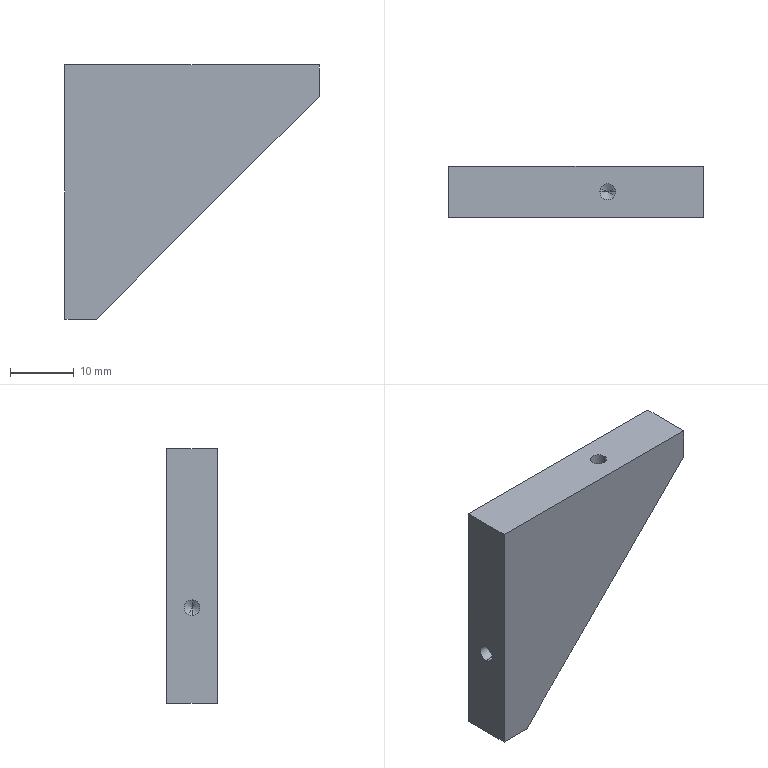Part | STEP file | PN_0010 | 1 solid | 15 faces | box 40 x 8 x 40 mm | volume 7824 mm3 | plane 7 | cylinder 4 | cone 4 | commonest cylinder face diameters 2.5 x4
STEP:
#1=CARTESIAN_POINT('',(0.,0.,0.));
#2=DIRECTION('',(0.,0.,1.));
#3=DIRECTION('',(1.,0.,0.));
#4=AXIS2_PLACEMENT_3D('',#1,#2,#3);
#5=CARTESIAN_POINT('',(-12.5,4.,-3.75));
#6=VERTEX_POINT('',#5);
#7=CARTESIAN_POINT('',(-20.,4.,-3.75));
#8=VERTEX_POINT('',#7);
#9=CARTESIAN_POINT('',(-20.,4.,-3.75));
#10=DIRECTION('',(-1.,0.,0.));
#11=VECTOR('',#10,1.);
#12=LINE('',#9,#11);
#13=CARTESIAN_POINT('',(-20.,4.,-5.));
#14=DIRECTION('',(-1.,0.,0.));
#15=DIRECTION('',(0.,0.,1.));
#16=AXIS2_PLACEMENT_3D('',#13,#14,#15);
#17=CYLINDRICAL_SURFACE('',#16,1.25);
#18=CARTESIAN_POINT('',(6.283,0.));
#19=DIRECTION('',(0.,1.));
#20=VECTOR('',#19,1.);
#21=LINE('',#18,#20);
#22=(GEOMETRIC_REPRESENTATION_CONTEXT(2)PARAMETRIC_REPRESENTATION_CONTEXT()REPRESENTATION_CONTEXT('',''));
#23=DEFINITIONAL_REPRESENTATION('',(#21),#22);
#24=PCURVE('',#17,#23);
#25=CARTESIAN_POINT('',(-20.,4.,-5.));
#26=DIRECTION('',(-1.,0.,0.));
#27=DIRECTION('',(0.,0.,1.));
#28=AXIS2_PLACEMENT_3D('',#25,#26,#27);
#29=CYLINDRICAL_SURFACE('',#28,1.25);
#30=CARTESIAN_POINT('',(0.,0.));
#31=DIRECTION('',(0.,1.));
#32=VECTOR('',#31,1.);
#33=LINE('',#30,#32);
#34=(GEOMETRIC_REPRESENTATION_CONTEXT(2)PARAMETRIC_REPRESENTATION_CONTEXT()REPRESENTATION_CONTEXT('',''));
#35=DEFINITIONAL_REPRESENTATION('',(#33),#34);
#36=PCURVE('',#29,#35);
#37=SURFACE_CURVE('',#12,(#24,#36),.PCURVE_S1.);
#38=EDGE_CURVE('',#6,#8,#37,.T.);
#39=ORIENTED_EDGE('',*,*,#38,.T.);
#40=CARTESIAN_POINT('',(-20.,4.,-6.25));
#41=VERTEX_POINT('',#40);
#42=CARTESIAN_POINT('',(-20.,4.,-5.));
#43=DIRECTION('',(-1.,0.,0.));
#44=DIRECTION('',(0.,0.,1.));
#45=AXIS2_PLACEMENT_3D('',#42,#43,#44);
#46=CIRCLE('',#45,1.25);
#47=CARTESIAN_POINT('',(0.,0.));
#48=DIRECTION('',(1.,0.));
#49=VECTOR('',#48,1.);
#50=LINE('',#47,#49);
#51=(GEOMETRIC_REPRESENTATION_CONTEXT(2)PARAMETRIC_REPRESENTATION_CONTEXT()REPRESENTATION_CONTEXT('',''));
#52=DEFINITIONAL_REPRESENTATION('',(#50),#51);
#53=PCURVE('',#17,#52);
#54=CARTESIAN_POINT('',(-20.,8.,-20.));
#55=DIRECTION('',(1.,0.,0.));
#56=DIRECTION('',(0.,0.,-1.));
#57=AXIS2_PLACEMENT_3D('',#54,#55,#56);
#58=PLANE('',#57);
#59=CARTESIAN_POINT('',(-16.25,-4.));
#60=CARTESIAN_POINT('',(-16.25,-1.835));
#61=CARTESIAN_POINT('',(-14.375,-2.917));
#62=CARTESIAN_POINT('',(-12.5,-4.));
#63=CARTESIAN_POINT('',(-14.375,-5.083));
#64=CARTESIAN_POINT('',(-16.25,-6.165));
#65=CARTESIAN_POINT('',(-16.25,-4.));
#66=(BOUNDED_CURVE()B_SPLINE_CURVE(2,(#59,#60,#61,#62,#63,#64,#65),.UNSPECIFIED.,.T.,.F.)B_SPLINE_CURVE_WITH_KNOTS((1,2,2,2,2,1),(-2.094,0.,2.094,4.189,6.283,8.378),.UNSPECIFIED.)CURVE()GEOMETRIC_REPRESENTATION_ITEM()RATIONAL_B_SPLINE_CURVE((1.,0.5,1.,0.5,1.,0.5,1.))REPRESENTATION_ITEM(''));
#67=(GEOMETRIC_REPRESENTATION_CONTEXT(2)PARAMETRIC_REPRESENTATION_CONTEXT()REPRESENTATION_CONTEXT('',''));
#68=DEFINITIONAL_REPRESENTATION('',(#66),#67);
#69=PCURVE('',#58,#68);
#70=SURFACE_CURVE('',#46,(#53,#69),.PCURVE_S1.);
#71=EDGE_CURVE('',#41,#8,#70,.T.);
#72=ORIENTED_EDGE('',*,*,#71,.F.);
#73=CARTESIAN_POINT('',(-12.5,4.,-6.25));
#74=VERTEX_POINT('',#73);
#75=CARTESIAN_POINT('',(-20.,4.,-6.25));
#76=DIRECTION('',(-1.,0.,0.));
#77=VECTOR('',#76,1.);
#78=LINE('',#75,#77);
#79=CARTESIAN_POINT('',(3.142,0.));
#80=DIRECTION('',(0.,1.));
#81=VECTOR('',#80,1.);
#82=LINE('',#79,#81);
#83=(GEOMETRIC_REPRESENTATION_CONTEXT(2)PARAMETRIC_REPRESENTATION_CONTEXT()REPRESENTATION_CONTEXT('',''));
#84=DEFINITIONAL_REPRESENTATION('',(#82),#83);
#85=PCURVE('',#17,#84);
#86=CARTESIAN_POINT('',(3.142,0.));
#87=DIRECTION('',(0.,1.));
#88=VECTOR('',#87,1.);
#89=LINE('',#86,#88);
#90=(GEOMETRIC_REPRESENTATION_CONTEXT(2)PARAMETRIC_REPRESENTATION_CONTEXT()REPRESENTATION_CONTEXT('',''));
#91=DEFINITIONAL_REPRESENTATION('',(#89),#90);
#92=PCURVE('',#29,#91);
#93=SURFACE_CURVE('',#78,(#85,#92),.PCURVE_S1.);
#94=EDGE_CURVE('',#74,#41,#93,.T.);
#95=ORIENTED_EDGE('',*,*,#94,.F.);
#96=CARTESIAN_POINT('',(-12.5,4.,-5.));
#97=DIRECTION('',(-1.,0.,0.));
#98=DIRECTION('',(0.,0.,1.));
#99=AXIS2_PLACEMENT_3D('',#96,#97,#98);
#100=CIRCLE('',#99,1.25);
#101=CARTESIAN_POINT('',(0.,-7.5));
#102=DIRECTION('',(1.,0.));
#103=VECTOR('',#102,1.);
#104=LINE('',#101,#103);
#105=(GEOMETRIC_REPRESENTATION_CONTEXT(2)PARAMETRIC_REPRESENTATION_CONTEXT()REPRESENTATION_CONTEXT('',''));
#106=DEFINITIONAL_REPRESENTATION('',(#104),#105);
#107=PCURVE('',#17,#106);
#108=CARTESIAN_POINT('',(-12.5,4.,-5.));
#109=DIRECTION('',(-1.,0.,0.));
#110=DIRECTION('',(0.,0.,1.));
#111=AXIS2_PLACEMENT_3D('',#108,#109,#110);
#112=CONICAL_SURFACE('',#111,1.25,1.03);
#113=CARTESIAN_POINT('',(0.,0.));
#114=DIRECTION('',(1.,0.));
#115=VECTOR('',#114,1.);
#116=LINE('',#113,#115);
#117=(GEOMETRIC_REPRESENTATION_CONTEXT(2)PARAMETRIC_REPRESENTATION_CONTEXT()REPRESENTATION_CONTEXT('',''));
#118=DEFINITIONAL_REPRESENTATION('',(#116),#117);
#119=PCURVE('',#112,#118);
#120=SURFACE_CURVE('',#100,(#107,#119),.PCURVE_S1.);
#121=EDGE_CURVE('',#74,#6,#120,.T.);
#122=ORIENTED_EDGE('',*,*,#121,.T.);
#123=EDGE_LOOP('',(#39,#72,#95,#122));
#124=FACE_BOUND('',#123,.F.);
#125=ADVANCED_FACE('',(#124),#17,.F.);
#126=ORIENTED_EDGE('',*,*,#121,.F.);
#127=CARTESIAN_POINT('',(-11.749,4.,-5.));
#128=VERTEX_POINT('',#127);
#129=CARTESIAN_POINT('',(-12.5,4.,-6.25));
#130=DIRECTION('',(-0.515,0.,-0.8572));
#131=VECTOR('',#130,1.);
#132=LINE('',#129,#131);
#133=CARTESIAN_POINT('',(3.142,0.));
#134=DIRECTION('',(0.,1.));
#135=VECTOR('',#134,1.);
#136=LINE('',#133,#135);
#137=(GEOMETRIC_REPRESENTATION_CONTEXT(2)PARAMETRIC_REPRESENTATION_CONTEXT()REPRESENTATION_CONTEXT('',''));
#138=DEFINITIONAL_REPRESENTATION('',(#136),#137);
#139=PCURVE('',#112,#138);
#140=CARTESIAN_POINT('',(-12.5,4.,-5.));
#141=DIRECTION('',(-1.,0.,0.));
#142=DIRECTION('',(0.,0.,1.));
#143=AXIS2_PLACEMENT_3D('',#140,#141,#142);
#144=CONICAL_SURFACE('',#143,1.25,1.03);
#145=CARTESIAN_POINT('',(3.142,0.));
#146=DIRECTION('',(0.,1.));
#147=VECTOR('',#146,1.);
#148=LINE('',#145,#147);
#149=(GEOMETRIC_REPRESENTATION_CONTEXT(2)PARAMETRIC_REPRESENTATION_CONTEXT()REPRESENTATION_CONTEXT('',''));
#150=DEFINITIONAL_REPRESENTATION('',(#148),#149);
#151=PCURVE('',#144,#150);
#152=SURFACE_CURVE('',#132,(#139,#151),.PCURVE_S1.);
#153=EDGE_CURVE('',#128,#74,#152,.T.);
#154=ORIENTED_EDGE('',*,*,#153,.F.);
#155=CARTESIAN_POINT('',(-12.5,4.,-3.75));
#156=DIRECTION('',(-0.515,0.,0.8572));
#157=VECTOR('',#156,1.);
#158=LINE('',#155,#157);
#159=CARTESIAN_POINT('',(6.283,0.));
#160=DIRECTION('',(0.,1.));
#161=VECTOR('',#160,1.);
#162=LINE('',#159,#161);
#163=(GEOMETRIC_REPRESENTATION_CONTEXT(2)PARAMETRIC_REPRESENTATION_CONTEXT()REPRESENTATION_CONTEXT('',''));
#164=DEFINITIONAL_REPRESENTATION('',(#162),#163);
#165=PCURVE('',#112,#164);
#166=CARTESIAN_POINT('',(0.,0.));
#167=DIRECTION('',(0.,1.));
#168=VECTOR('',#167,1.);
#169=LINE('',#166,#168);
#170=(GEOMETRIC_REPRESENTATION_CONTEXT(2)PARAMETRIC_REPRESENTATION_CONTEXT()REPRESENTATION_CONTEXT('',''));
#171=DEFINITIONAL_REPRESENTATION('',(#169),#170);
#172=PCURVE('',#144,#171);
#173=SURFACE_CURVE('',#158,(#165,#172),.PCURVE_S1.);
#174=EDGE_CURVE('',#128,#6,#173,.T.);
#175=ORIENTED_EDGE('',*,*,#174,.T.);
#176=EDGE_LOOP('',(#126,#154,#175));
#177=FACE_BOUND('',#176,.F.);
#178=ADVANCED_FACE('',(#177),#112,.F.);
#179=CARTESIAN_POINT('',(6.25,4.,12.5));
#180=VERTEX_POINT('',#179);
#181=CARTESIAN_POINT('',(6.25,4.,20.));
#182=VERTEX_POINT('',#181);
#183=CARTESIAN_POINT('',(6.25,4.,20.));
#184=DIRECTION('',(0.,0.,1.));
#185=VECTOR('',#184,1.);
#186=LINE('',#183,#185);
#187=CARTESIAN_POINT('',(5.,4.,20.));
#188=DIRECTION('',(0.,0.,1.));
#189=DIRECTION('',(1.,0.,0.));
#190=AXIS2_PLACEMENT_3D('',#187,#188,#189);
#191=CYLINDRICAL_SURFACE('',#190,1.25);
#192=CARTESIAN_POINT('',(6.283,0.));
#193=DIRECTION('',(0.,1.));
#194=VECTOR('',#193,1.);
#195=LINE('',#192,#194);
#196=(GEOMETRIC_REPRESENTATION_CONTEXT(2)PARAMETRIC_REPRESENTATION_CONTEXT()REPRESENTATION_CONTEXT('',''));
#197=DEFINITIONAL_REPRESENTATION('',(#195),#196);
#198=PCURVE('',#191,#197);
#199=CARTESIAN_POINT('',(5.,4.,20.));
#200=DIRECTION('',(0.,0.,1.));
#201=DIRECTION('',(1.,0.,0.));
#202=AXIS2_PLACEMENT_3D('',#199,#200,#201);
#203=CYLINDRICAL_SURFACE('',#202,1.25);
#204=CARTESIAN_POINT('',(0.,0.));
#205=DIRECTION('',(0.,1.));
#206=VECTOR('',#205,1.);
#207=LINE('',#204,#206);
#208=(GEOMETRIC_REPRESENTATION_CONTEXT(2)PARAMETRIC_REPRESENTATION_CONTEXT()REPRESENTATION_CONTEXT('',''));
#209=DEFINITIONAL_REPRESENTATION('',(#207),#208);
#210=PCURVE('',#203,#209);
#211=SURFACE_CURVE('',#186,(#198,#210),.PCURVE_S1.);
#212=EDGE_CURVE('',#180,#182,#211,.T.);
#213=ORIENTED_EDGE('',*,*,#212,.T.);
#214=CARTESIAN_POINT('',(3.75,4.,20.));
#215=VERTEX_POINT('',#214);
#216=CARTESIAN_POINT('',(5.,4.,20.));
#217=DIRECTION('',(0.,0.,1.));
#218=DIRECTION('',(1.,0.,0.));
#219=AXIS2_PLACEMENT_3D('',#216,#217,#218);
#220=CIRCLE('',#219,1.25);
#221=CARTESIAN_POINT('',(0.,0.));
#222=DIRECTION('',(1.,0.));
#223=VECTOR('',#222,1.);
#224=LINE('',#221,#223);
#225=(GEOMETRIC_REPRESENTATION_CONTEXT(2)PARAMETRIC_REPRESENTATION_CONTEXT()REPRESENTATION_CONTEXT('',''));
#226=DEFINITIONAL_REPRESENTATION('',(#224),#225);
#227=PCURVE('',#191,#226);
#228=CARTESIAN_POINT('',(-20.,8.,20.));
#229=DIRECTION('',(0.,0.,-1.));
#230=DIRECTION('',(-1.,0.,0.));
#231=AXIS2_PLACEMENT_3D('',#228,#229,#230);
#232=PLANE('',#231);
#233=CARTESIAN_POINT('',(-26.25,-4.));
#234=CARTESIAN_POINT('',(-26.25,-1.835));
#235=CARTESIAN_POINT('',(-24.375,-2.917));
#236=CARTESIAN_POINT('',(-22.5,-4.));
#237=CARTESIAN_POINT('',(-24.375,-5.083));
#238=CARTESIAN_POINT('',(-26.25,-6.165));
#239=CARTESIAN_POINT('',(-26.25,-4.));
#240=(BOUNDED_CURVE()B_SPLINE_CURVE(2,(#233,#234,#235,#236,#237,#238,#239),.UNSPECIFIED.,.T.,.F.)B_SPLINE_CURVE_WITH_KNOTS((1,2,2,2,2,1),(-2.094,0.,2.094,4.189,6.283,8.378),.UNSPECIFIED.)CURVE()GEOMETRIC_REPRESENTATION_ITEM()RATIONAL_B_SPLINE_CURVE((1.,0.5,1.,0.5,1.,0.5,1.))REPRESENTATION_ITEM(''));
#241=(GEOMETRIC_REPRESENTATION_CONTEXT(2)PARAMETRIC_REPRESENTATION_CONTEXT()REPRESENTATION_CONTEXT('',''));
#242=DEFINITIONAL_REPRESENTATION('',(#240),#241);
#243=PCURVE('',#232,#242);
#244=SURFACE_CURVE('',#220,(#227,#243),.PCURVE_S1.);
#245=EDGE_CURVE('',#215,#182,#244,.T.);
#246=ORIENTED_EDGE('',*,*,#245,.F.);
#247=CARTESIAN_POINT('',(3.75,4.,12.5));
#248=VERTEX_POINT('',#247);
#249=CARTESIAN_POINT('',(3.75,4.,20.));
#250=DIRECTION('',(0.,0.,1.));
#251=VECTOR('',#250,1.);
#252=LINE('',#249,#251);
#253=CARTESIAN_POINT('',(3.142,0.));
#254=DIRECTION('',(0.,1.));
#255=VECTOR('',#254,1.);
#256=LINE('',#253,#255);
#257=(GEOMETRIC_REPRESENTATION_CONTEXT(2)PARAMETRIC_REPRESENTATION_CONTEXT()REPRESENTATION_CONTEXT('',''));
#258=DEFINITIONAL_REPRESENTATION('',(#256),#257);
#259=PCURVE('',#191,#258);
#260=CARTESIAN_POINT('',(3.142,0.));
#261=DIRECTION('',(0.,1.));
#262=VECTOR('',#261,1.);
#263=LINE('',#260,#262);
#264=(GEOMETRIC_REPRESENTATION_CONTEXT(2)PARAMETRIC_REPRESENTATION_CONTEXT()REPRESENTATION_CONTEXT('',''));
#265=DEFINITIONAL_REPRESENTATION('',(#263),#264);
#266=PCURVE('',#203,#265);
#267=SURFACE_CURVE('',#252,(#259,#266),.PCURVE_S1.);
#268=EDGE_CURVE('',#248,#215,#267,.T.);
#269=ORIENTED_EDGE('',*,*,#268,.F.);
#270=CARTESIAN_POINT('',(5.,4.,12.5));
#271=DIRECTION('',(0.,0.,1.));
#272=DIRECTION('',(1.,0.,0.));
#273=AXIS2_PLACEMENT_3D('',#270,#271,#272);
#274=CIRCLE('',#273,1.25);
#275=CARTESIAN_POINT('',(0.,-7.5));
#276=DIRECTION('',(1.,0.));
#277=VECTOR('',#276,1.);
#278=LINE('',#275,#277);
#279=(GEOMETRIC_REPRESENTATION_CONTEXT(2)PARAMETRIC_REPRESENTATION_CONTEXT()REPRESENTATION_CONTEXT('',''));
#280=DEFINITIONAL_REPRESENTATION('',(#278),#279);
#281=PCURVE('',#191,#280);
#282=CARTESIAN_POINT('',(5.,4.,12.5));
#283=DIRECTION('',(0.,0.,1.));
#284=DIRECTION('',(1.,0.,0.));
#285=AXIS2_PLACEMENT_3D('',#282,#283,#284);
#286=CONICAL_SURFACE('',#285,1.25,1.03);
#287=CARTESIAN_POINT('',(0.,0.));
#288=DIRECTION('',(1.,0.));
#289=VECTOR('',#288,1.);
#290=LINE('',#287,#289);
#291=(GEOMETRIC_REPRESENTATION_CONTEXT(2)PARAMETRIC_REPRESENTATION_CONTEXT()REPRESENTATION_CONTEXT('',''));
#292=DEFINITIONAL_REPRESENTATION('',(#290),#291);
#293=PCURVE('',#286,#292);
#294=SURFACE_CURVE('',#274,(#281,#293),.PCURVE_S1.);
#295=EDGE_CURVE('',#248,#180,#294,.T.);
#296=ORIENTED_EDGE('',*,*,#295,.T.);
#297=EDGE_LOOP('',(#213,#246,#269,#296));
#298=FACE_BOUND('',#297,.F.);
#299=ADVANCED_FACE('',(#298),#191,.F.);
#300=ORIENTED_EDGE('',*,*,#295,.F.);
#301=CARTESIAN_POINT('',(5.,4.,11.749));
#302=VERTEX_POINT('',#301);
#303=CARTESIAN_POINT('',(3.75,4.,12.5));
#304=DIRECTION('',(-0.8572,0.,0.515));
#305=VECTOR('',#304,1.);
#306=LINE('',#303,#305);
#307=CARTESIAN_POINT('',(3.142,0.));
#308=DIRECTION('',(0.,1.));
#309=VECTOR('',#308,1.);
#310=LINE('',#307,#309);
#311=(GEOMETRIC_REPRESENTATION_CONTEXT(2)PARAMETRIC_REPRESENTATION_CONTEXT()REPRESENTATION_CONTEXT('',''));
#312=DEFINITIONAL_REPRESENTATION('',(#310),#311);
#313=PCURVE('',#286,#312);
#314=CARTESIAN_POINT('',(5.,4.,12.5));
#315=DIRECTION('',(0.,0.,1.));
#316=DIRECTION('',(1.,0.,0.));
#317=AXIS2_PLACEMENT_3D('',#314,#315,#316);
#318=CONICAL_SURFACE('',#317,1.25,1.03);
#319=CARTESIAN_POINT('',(3.142,0.));
#320=DIRECTION('',(0.,1.));
#321=VECTOR('',#320,1.);
#322=LINE('',#319,#321);
#323=(GEOMETRIC_REPRESENTATION_CONTEXT(2)PARAMETRIC_REPRESENTATION_CONTEXT()REPRESENTATION_CONTEXT('',''));
#324=DEFINITIONAL_REPRESENTATION('',(#322),#323);
#325=PCURVE('',#318,#324);
#326=SURFACE_CURVE('',#306,(#313,#325),.PCURVE_S1.);
#327=EDGE_CURVE('',#302,#248,#326,.T.);
#328=ORIENTED_EDGE('',*,*,#327,.F.);
#329=CARTESIAN_POINT('',(6.25,4.,12.5));
#330=DIRECTION('',(0.8572,0.,0.515));
#331=VECTOR('',#330,1.);
#332=LINE('',#329,#331);
#333=CARTESIAN_POINT('',(6.283,0.));
#334=DIRECTION('',(0.,1.));
#335=VECTOR('',#334,1.);
#336=LINE('',#333,#335);
#337=(GEOMETRIC_REPRESENTATION_CONTEXT(2)PARAMETRIC_REPRESENTATION_CONTEXT()REPRESENTATION_CONTEXT('',''));
#338=DEFINITIONAL_REPRESENTATION('',(#336),#337);
#339=PCURVE('',#286,#338);
#340=CARTESIAN_POINT('',(0.,0.));
#341=DIRECTION('',(0.,1.));
#342=VECTOR('',#341,1.);
#343=LINE('',#340,#342);
#344=(GEOMETRIC_REPRESENTATION_CONTEXT(2)PARAMETRIC_REPRESENTATION_CONTEXT()REPRESENTATION_CONTEXT('',''));
#345=DEFINITIONAL_REPRESENTATION('',(#343),#344);
#346=PCURVE('',#318,#345);
#347=SURFACE_CURVE('',#332,(#339,#346),.PCURVE_S1.);
#348=EDGE_CURVE('',#302,#180,#347,.T.);
#349=ORIENTED_EDGE('',*,*,#348,.T.);
#350=EDGE_LOOP('',(#300,#328,#349));
#351=FACE_BOUND('',#350,.F.);
#352=ADVANCED_FACE('',(#351),#286,.F.);
#353=CARTESIAN_POINT('',(20.,0.,20.));
#354=VERTEX_POINT('',#353);
#355=CARTESIAN_POINT('',(20.,0.,15.));
#356=VERTEX_POINT('',#355);
#357=CARTESIAN_POINT('',(20.,0.,-20.));
#358=DIRECTION('',(0.,0.,-1.));
#359=VECTOR('',#358,1.);
#360=LINE('',#357,#359);
#361=CARTESIAN_POINT('',(20.,8.,-20.));
#362=DIRECTION('',(-1.,0.,0.));
#363=DIRECTION('',(0.,0.,1.));
#364=AXIS2_PLACEMENT_3D('',#361,#362,#363);
#365=PLANE('',#364);
#366=CARTESIAN_POINT('',(0.,-8.));
#367=DIRECTION('',(-1.,0.));
#368=VECTOR('',#367,1.);
#369=LINE('',#366,#368);
#370=(GEOMETRIC_REPRESENTATION_CONTEXT(2)PARAMETRIC_REPRESENTATION_CONTEXT()REPRESENTATION_CONTEXT('',''));
#371=DEFINITIONAL_REPRESENTATION('',(#369),#370);
#372=PCURVE('',#365,#371);
#373=CARTESIAN_POINT('',(0.,0.,0.));
#374=DIRECTION('',(0.,1.,0.));
#375=DIRECTION('',(0.,0.,1.));
#376=AXIS2_PLACEMENT_3D('',#373,#374,#375);
#377=PLANE('',#376);
#378=CARTESIAN_POINT('',(-20.,20.));
#379=DIRECTION('',(-1.,0.));
#380=VECTOR('',#379,1.);
#381=LINE('',#378,#380);
#382=(GEOMETRIC_REPRESENTATION_CONTEXT(2)PARAMETRIC_REPRESENTATION_CONTEXT()REPRESENTATION_CONTEXT('',''));
#383=DEFINITIONAL_REPRESENTATION('',(#381),#382);
#384=PCURVE('',#377,#383);
#385=SURFACE_CURVE('',#360,(#372,#384),.PCURVE_S1.);
#386=EDGE_CURVE('',#354,#356,#385,.T.);
#387=ORIENTED_EDGE('',*,*,#386,.T.);
#388=CARTESIAN_POINT('',(20.,8.,15.));
#389=VERTEX_POINT('',#388);
#390=CARTESIAN_POINT('',(20.,0.,15.));
#391=DIRECTION('',(0.,1.,0.));
#392=VECTOR('',#391,1.);
#393=LINE('',#390,#392);
#394=CARTESIAN_POINT('',(35.,-8.));
#395=DIRECTION('',(0.,1.));
#396=VECTOR('',#395,1.);
#397=LINE('',#394,#396);
#398=(GEOMETRIC_REPRESENTATION_CONTEXT(2)PARAMETRIC_REPRESENTATION_CONTEXT()REPRESENTATION_CONTEXT('',''));
#399=DEFINITIONAL_REPRESENTATION('',(#397),#398);
#400=PCURVE('',#365,#399);
#401=CARTESIAN_POINT('',(20.,0.,15.));
#402=DIRECTION('',(-0.7071,0.,0.7071));
#403=DIRECTION('',(0.7071,0.,0.7071));
#404=AXIS2_PLACEMENT_3D('',#401,#402,#403);
#405=PLANE('',#404);
#406=CARTESIAN_POINT('',(0.,0.));
#407=DIRECTION('',(0.,1.));
#408=VECTOR('',#407,1.);
#409=LINE('',#406,#408);
#410=(GEOMETRIC_REPRESENTATION_CONTEXT(2)PARAMETRIC_REPRESENTATION_CONTEXT()REPRESENTATION_CONTEXT('',''));
#411=DEFINITIONAL_REPRESENTATION('',(#409),#410);
#412=PCURVE('',#405,#411);
#413=SURFACE_CURVE('',#393,(#400,#412),.PCURVE_S1.);
#414=EDGE_CURVE('',#356,#389,#413,.T.);
#415=ORIENTED_EDGE('',*,*,#414,.T.);
#416=CARTESIAN_POINT('',(20.,8.,20.));
#417=VERTEX_POINT('',#416);
#418=CARTESIAN_POINT('',(20.,8.,-20.));
#419=DIRECTION('',(0.,0.,-1.));
#420=VECTOR('',#419,1.);
#421=LINE('',#418,#420);
#422=CARTESIAN_POINT('',(0.,0.));
#423=DIRECTION('',(-1.,0.));
#424=VECTOR('',#423,1.);
#425=LINE('',#422,#424);
#426=(GEOMETRIC_REPRESENTATION_CONTEXT(2)PARAMETRIC_REPRESENTATION_CONTEXT()REPRESENTATION_CONTEXT('',''));
#427=DEFINITIONAL_REPRESENTATION('',(#425),#426);
#428=PCURVE('',#365,#427);
#429=CARTESIAN_POINT('',(0.,8.,0.));
#430=DIRECTION('',(0.,1.,0.));
#431=DIRECTION('',(0.,0.,1.));
#432=AXIS2_PLACEMENT_3D('',#429,#430,#431);
#433=PLANE('',#432);
#434=CARTESIAN_POINT('',(-20.,20.));
#435=DIRECTION('',(-1.,0.));
#436=VECTOR('',#435,1.);
#437=LINE('',#434,#436);
#438=(GEOMETRIC_REPRESENTATION_CONTEXT(2)PARAMETRIC_REPRESENTATION_CONTEXT()REPRESENTATION_CONTEXT('',''));
#439=DEFINITIONAL_REPRESENTATION('',(#437),#438);
#440=PCURVE('',#433,#439);
#441=SURFACE_CURVE('',#421,(#428,#440),.PCURVE_S1.);
#442=EDGE_CURVE('',#417,#389,#441,.T.);
#443=ORIENTED_EDGE('',*,*,#442,.F.);
#444=CARTESIAN_POINT('',(20.,8.,20.));
#445=DIRECTION('',(0.,-1.,0.));
#446=VECTOR('',#445,1.);
#447=LINE('',#444,#446);
#448=CARTESIAN_POINT('',(40.,0.));
#449=DIRECTION('',(0.,-1.));
#450=VECTOR('',#449,1.);
#451=LINE('',#448,#450);
#452=(GEOMETRIC_REPRESENTATION_CONTEXT(2)PARAMETRIC_REPRESENTATION_CONTEXT()REPRESENTATION_CONTEXT('',''));
#453=DEFINITIONAL_REPRESENTATION('',(#451),#452);
#454=PCURVE('',#365,#453);
#455=CARTESIAN_POINT('',(-40.,0.));
#456=DIRECTION('',(0.,-1.));
#457=VECTOR('',#456,1.);
#458=LINE('',#455,#457);
#459=(GEOMETRIC_REPRESENTATION_CONTEXT(2)PARAMETRIC_REPRESENTATION_CONTEXT()REPRESENTATION_CONTEXT('',''));
#460=DEFINITIONAL_REPRESENTATION('',(#458),#459);
#461=PCURVE('',#232,#460);
#462=SURFACE_CURVE('',#447,(#454,#461),.PCURVE_S1.);
#463=EDGE_CURVE('',#417,#354,#462,.T.);
#464=ORIENTED_EDGE('',*,*,#463,.T.);
#465=EDGE_LOOP('',(#387,#415,#443,#464));
#466=FACE_BOUND('',#465,.T.);
#467=ADVANCED_FACE('',(#466),#365,.F.);
#468=CARTESIAN_POINT('',(-15.,8.,-20.));
#469=VERTEX_POINT('',#468);
#470=CARTESIAN_POINT('',(-20.,8.,-20.));
#471=VERTEX_POINT('',#470);
#472=CARTESIAN_POINT('',(-20.,8.,-20.));
#473=DIRECTION('',(-1.,0.,0.));
#474=VECTOR('',#473,1.);
#475=LINE('',#472,#474);
#476=CARTESIAN_POINT('',(-20.,8.,-20.));
#477=DIRECTION('',(0.,0.,1.));
#478=DIRECTION('',(1.,0.,0.));
#479=AXIS2_PLACEMENT_3D('',#476,#477,#478);
#480=PLANE('',#479);
#481=CARTESIAN_POINT('',(0.,0.));
#482=DIRECTION('',(-1.,0.));
#483=VECTOR('',#482,1.);
#484=LINE('',#481,#483);
#485=(GEOMETRIC_REPRESENTATION_CONTEXT(2)PARAMETRIC_REPRESENTATION_CONTEXT()REPRESENTATION_CONTEXT('',''));
#486=DEFINITIONAL_REPRESENTATION('',(#484),#485);
#487=PCURVE('',#480,#486);
#488=CARTESIAN_POINT('',(-20.,-20.));
#489=DIRECTION('',(0.,-1.));
#490=VECTOR('',#489,1.);
#491=LINE('',#488,#490);
#492=(GEOMETRIC_REPRESENTATION_CONTEXT(2)PARAMETRIC_REPRESENTATION_CONTEXT()REPRESENTATION_CONTEXT('',''));
#493=DEFINITIONAL_REPRESENTATION('',(#491),#492);
#494=PCURVE('',#433,#493);
#495=SURFACE_CURVE('',#475,(#487,#494),.PCURVE_S1.);
#496=EDGE_CURVE('',#469,#471,#495,.T.);
#497=ORIENTED_EDGE('',*,*,#496,.F.);
#498=CARTESIAN_POINT('',(-15.,0.,-20.));
#499=VERTEX_POINT('',#498);
#500=CARTESIAN_POINT('',(-15.,0.,-20.));
#501=DIRECTION('',(0.,1.,0.));
#502=VECTOR('',#501,1.);
#503=LINE('',#500,#502);
#504=CARTESIAN_POINT('',(5.,-8.));
#505=DIRECTION('',(0.,1.));
#506=VECTOR('',#505,1.);
#507=LINE('',#504,#506);
#508=(GEOMETRIC_REPRESENTATION_CONTEXT(2)PARAMETRIC_REPRESENTATION_CONTEXT()REPRESENTATION_CONTEXT('',''));
#509=DEFINITIONAL_REPRESENTATION('',(#507),#508);
#510=PCURVE('',#480,#509);
#511=CARTESIAN_POINT('',(-49.497,0.));
#512=DIRECTION('',(0.,1.));
#513=VECTOR('',#512,1.);
#514=LINE('',#511,#513);
#515=(GEOMETRIC_REPRESENTATION_CONTEXT(2)PARAMETRIC_REPRESENTATION_CONTEXT()REPRESENTATION_CONTEXT('',''));
#516=DEFINITIONAL_REPRESENTATION('',(#514),#515);
#517=PCURVE('',#405,#516);
#518=SURFACE_CURVE('',#503,(#510,#517),.PCURVE_S1.);
#519=EDGE_CURVE('',#499,#469,#518,.T.);
#520=ORIENTED_EDGE('',*,*,#519,.F.);
#521=CARTESIAN_POINT('',(-20.,0.,-20.));
#522=VERTEX_POINT('',#521);
#523=CARTESIAN_POINT('',(-20.,0.,-20.));
#524=DIRECTION('',(-1.,0.,0.));
#525=VECTOR('',#524,1.);
#526=LINE('',#523,#525);
#527=CARTESIAN_POINT('',(0.,-8.));
#528=DIRECTION('',(-1.,0.));
#529=VECTOR('',#528,1.);
#530=LINE('',#527,#529);
#531=(GEOMETRIC_REPRESENTATION_CONTEXT(2)PARAMETRIC_REPRESENTATION_CONTEXT()REPRESENTATION_CONTEXT('',''));
#532=DEFINITIONAL_REPRESENTATION('',(#530),#531);
#533=PCURVE('',#480,#532);
#534=CARTESIAN_POINT('',(-20.,-20.));
#535=DIRECTION('',(0.,-1.));
#536=VECTOR('',#535,1.);
#537=LINE('',#534,#536);
#538=(GEOMETRIC_REPRESENTATION_CONTEXT(2)PARAMETRIC_REPRESENTATION_CONTEXT()REPRESENTATION_CONTEXT('',''));
#539=DEFINITIONAL_REPRESENTATION('',(#537),#538);
#540=PCURVE('',#377,#539);
#541=SURFACE_CURVE('',#526,(#533,#540),.PCURVE_S1.);
#542=EDGE_CURVE('',#499,#522,#541,.T.);
#543=ORIENTED_EDGE('',*,*,#542,.T.);
#544=CARTESIAN_POINT('',(-20.,8.,-20.));
#545=DIRECTION('',(0.,-1.,0.));
#546=VECTOR('',#545,1.);
#547=LINE('',#544,#546);
#548=CARTESIAN_POINT('',(0.,0.));
#549=DIRECTION('',(0.,-1.));
#550=VECTOR('',#549,1.);
#551=LINE('',#548,#550);
#552=(GEOMETRIC_REPRESENTATION_CONTEXT(2)PARAMETRIC_REPRESENTATION_CONTEXT()REPRESENTATION_CONTEXT('',''));
#553=DEFINITIONAL_REPRESENTATION('',(#551),#552);
#554=PCURVE('',#480,#553);
#555=CARTESIAN_POINT('',(0.,0.));
#556=DIRECTION('',(0.,-1.));
#557=VECTOR('',#556,1.);
#558=LINE('',#555,#557);
#559=(GEOMETRIC_REPRESENTATION_CONTEXT(2)PARAMETRIC_REPRESENTATION_CONTEXT()REPRESENTATION_CONTEXT('',''));
#560=DEFINITIONAL_REPRESENTATION('',(#558),#559);
#561=PCURVE('',#58,#560);
#562=SURFACE_CURVE('',#547,(#554,#561),.PCURVE_S1.);
#563=EDGE_CURVE('',#471,#522,#562,.T.);
#564=ORIENTED_EDGE('',*,*,#563,.F.);
#565=EDGE_LOOP('',(#497,#520,#543,#564));
#566=FACE_BOUND('',#565,.T.);
#567=ADVANCED_FACE('',(#566),#480,.F.);
#568=CARTESIAN_POINT('',(-20.,4.,-5.));
#569=DIRECTION('',(-1.,0.,0.));
#570=DIRECTION('',(0.,0.,1.));
#571=AXIS2_PLACEMENT_3D('',#568,#569,#570);
#572=CIRCLE('',#571,1.25);
#573=CARTESIAN_POINT('',(-16.25,-4.));
#574=CARTESIAN_POINT('',(-16.25,-1.835));
#575=CARTESIAN_POINT('',(-14.375,-2.917));
#576=CARTESIAN_POINT('',(-12.5,-4.));
#577=CARTESIAN_POINT('',(-14.375,-5.083));
#578=CARTESIAN_POINT('',(-16.25,-6.165));
#579=CARTESIAN_POINT('',(-16.25,-4.));
#580=(BOUNDED_CURVE()B_SPLINE_CURVE(2,(#573,#574,#575,#576,#577,#578,#579),.UNSPECIFIED.,.T.,.F.)B_SPLINE_CURVE_WITH_KNOTS((1,2,2,2,2,1),(-2.094,0.,2.094,4.189,6.283,8.378),.UNSPECIFIED.)CURVE()GEOMETRIC_REPRESENTATION_ITEM()RATIONAL_B_SPLINE_CURVE((1.,0.5,1.,0.5,1.,0.5,1.))REPRESENTATION_ITEM(''));
#581=(GEOMETRIC_REPRESENTATION_CONTEXT(2)PARAMETRIC_REPRESENTATION_CONTEXT()REPRESENTATION_CONTEXT('',''));
#582=DEFINITIONAL_REPRESENTATION('',(#580),#581);
#583=PCURVE('',#58,#582);
#584=CARTESIAN_POINT('',(0.,0.));
#585=DIRECTION('',(1.,0.));
#586=VECTOR('',#585,1.);
#587=LINE('',#584,#586);
#588=(GEOMETRIC_REPRESENTATION_CONTEXT(2)PARAMETRIC_REPRESENTATION_CONTEXT()REPRESENTATION_CONTEXT('',''));
#589=DEFINITIONAL_REPRESENTATION('',(#587),#588);
#590=PCURVE('',#29,#589);
#591=SURFACE_CURVE('',#572,(#583,#590),.PCURVE_S1.);
#592=EDGE_CURVE('',#8,#41,#591,.T.);
#593=ORIENTED_EDGE('',*,*,#592,.F.);
#594=ORIENTED_EDGE('',*,*,#71,.F.);
#595=EDGE_LOOP('',(#593,#594));
#596=FACE_BOUND('',#595,.T.);
#597=CARTESIAN_POINT('',(-20.,0.,20.));
#598=VERTEX_POINT('',#597);
#599=CARTESIAN_POINT('',(-20.,0.,-20.));
#600=DIRECTION('',(0.,0.,1.));
#601=VECTOR('',#600,1.);
#602=LINE('',#599,#601);
#603=CARTESIAN_POINT('',(0.,-8.));
#604=DIRECTION('',(-1.,0.));
#605=VECTOR('',#604,1.);
#606=LINE('',#603,#605);
#607=(GEOMETRIC_REPRESENTATION_CONTEXT(2)PARAMETRIC_REPRESENTATION_CONTEXT()REPRESENTATION_CONTEXT('',''));
#608=DEFINITIONAL_REPRESENTATION('',(#606),#607);
#609=PCURVE('',#58,#608);
#610=CARTESIAN_POINT('',(-20.,-20.));
#611=DIRECTION('',(1.,0.));
#612=VECTOR('',#611,1.);
#613=LINE('',#610,#612);
#614=(GEOMETRIC_REPRESENTATION_CONTEXT(2)PARAMETRIC_REPRESENTATION_CONTEXT()REPRESENTATION_CONTEXT('',''));
#615=DEFINITIONAL_REPRESENTATION('',(#613),#614);
#616=PCURVE('',#377,#615);
#617=SURFACE_CURVE('',#602,(#609,#616),.PCURVE_S1.);
#618=EDGE_CURVE('',#522,#598,#617,.T.);
#619=ORIENTED_EDGE('',*,*,#618,.T.);
#620=CARTESIAN_POINT('',(-20.,8.,20.));
#621=VERTEX_POINT('',#620);
#622=CARTESIAN_POINT('',(-20.,8.,20.));
#623=DIRECTION('',(0.,-1.,0.));
#624=VECTOR('',#623,1.);
#625=LINE('',#622,#624);
#626=CARTESIAN_POINT('',(-40.,0.));
#627=DIRECTION('',(0.,-1.));
#628=VECTOR('',#627,1.);
#629=LINE('',#626,#628);
#630=(GEOMETRIC_REPRESENTATION_CONTEXT(2)PARAMETRIC_REPRESENTATION_CONTEXT()REPRESENTATION_CONTEXT('',''));
#631=DEFINITIONAL_REPRESENTATION('',(#629),#630);
#632=PCURVE('',#58,#631);
#633=CARTESIAN_POINT('',(0.,0.));
#634=DIRECTION('',(0.,-1.));
#635=VECTOR('',#634,1.);
#636=LINE('',#633,#635);
#637=(GEOMETRIC_REPRESENTATION_CONTEXT(2)PARAMETRIC_REPRESENTATION_CONTEXT()REPRESENTATION_CONTEXT('',''));
#638=DEFINITIONAL_REPRESENTATION('',(#636),#637);
#639=PCURVE('',#232,#638);
#640=SURFACE_CURVE('',#625,(#632,#639),.PCURVE_S1.);
#641=EDGE_CURVE('',#621,#598,#640,.T.);
#642=ORIENTED_EDGE('',*,*,#641,.F.);
#643=CARTESIAN_POINT('',(-20.,8.,-20.));
#644=DIRECTION('',(0.,0.,1.));
#645=VECTOR('',#644,1.);
#646=LINE('',#643,#645);
#647=CARTESIAN_POINT('',(0.,0.));
#648=DIRECTION('',(-1.,0.));
#649=VECTOR('',#648,1.);
#650=LINE('',#647,#649);
#651=(GEOMETRIC_REPRESENTATION_CONTEXT(2)PARAMETRIC_REPRESENTATION_CONTEXT()REPRESENTATION_CONTEXT('',''));
#652=DEFINITIONAL_REPRESENTATION('',(#650),#651);
#653=PCURVE('',#58,#652);
#654=CARTESIAN_POINT('',(-20.,-20.));
#655=DIRECTION('',(1.,0.));
#656=VECTOR('',#655,1.);
#657=LINE('',#654,#656);
#658=(GEOMETRIC_REPRESENTATION_CONTEXT(2)PARAMETRIC_REPRESENTATION_CONTEXT()REPRESENTATION_CONTEXT('',''));
#659=DEFINITIONAL_REPRESENTATION('',(#657),#658);
#660=PCURVE('',#433,#659);
#661=SURFACE_CURVE('',#646,(#653,#660),.PCURVE_S1.);
#662=EDGE_CURVE('',#471,#621,#661,.T.);
#663=ORIENTED_EDGE('',*,*,#662,.F.);
#664=ORIENTED_EDGE('',*,*,#563,.T.);
#665=EDGE_LOOP('',(#619,#642,#663,#664));
#666=FACE_BOUND('',#665,.T.);
#667=ADVANCED_FACE('',(#596,#666),#58,.F.);
#668=CARTESIAN_POINT('',(5.,4.,20.));
#669=DIRECTION('',(0.,0.,1.));
#670=DIRECTION('',(1.,0.,0.));
#671=AXIS2_PLACEMENT_3D('',#668,#669,#670);
#672=CIRCLE('',#671,1.25);
#673=CARTESIAN_POINT('',(-26.25,-4.));
#674=CARTESIAN_POINT('',(-26.25,-1.835));
#675=CARTESIAN_POINT('',(-24.375,-2.917));
#676=CARTESIAN_POINT('',(-22.5,-4.));
#677=CARTESIAN_POINT('',(-24.375,-5.083));
#678=CARTESIAN_POINT('',(-26.25,-6.165));
#679=CARTESIAN_POINT('',(-26.25,-4.));
#680=(BOUNDED_CURVE()B_SPLINE_CURVE(2,(#673,#674,#675,#676,#677,#678,#679),.UNSPECIFIED.,.T.,.F.)B_SPLINE_CURVE_WITH_KNOTS((1,2,2,2,2,1),(-2.094,0.,2.094,4.189,6.283,8.378),.UNSPECIFIED.)CURVE()GEOMETRIC_REPRESENTATION_ITEM()RATIONAL_B_SPLINE_CURVE((1.,0.5,1.,0.5,1.,0.5,1.))REPRESENTATION_ITEM(''));
#681=(GEOMETRIC_REPRESENTATION_CONTEXT(2)PARAMETRIC_REPRESENTATION_CONTEXT()REPRESENTATION_CONTEXT('',''));
#682=DEFINITIONAL_REPRESENTATION('',(#680),#681);
#683=PCURVE('',#232,#682);
#684=CARTESIAN_POINT('',(0.,0.));
#685=DIRECTION('',(1.,0.));
#686=VECTOR('',#685,1.);
#687=LINE('',#684,#686);
#688=(GEOMETRIC_REPRESENTATION_CONTEXT(2)PARAMETRIC_REPRESENTATION_CONTEXT()REPRESENTATION_CONTEXT('',''));
#689=DEFINITIONAL_REPRESENTATION('',(#687),#688);
#690=PCURVE('',#203,#689);
#691=SURFACE_CURVE('',#672,(#683,#690),.PCURVE_S1.);
#692=EDGE_CURVE('',#182,#215,#691,.T.);
#693=ORIENTED_EDGE('',*,*,#692,.F.);
#694=ORIENTED_EDGE('',*,*,#245,.F.);
#695=EDGE_LOOP('',(#693,#694));
#696=FACE_BOUND('',#695,.T.);
#697=CARTESIAN_POINT('',(-20.,0.,20.));
#698=DIRECTION('',(1.,0.,0.));
#699=VECTOR('',#698,1.);
#700=LINE('',#697,#699);
#701=CARTESIAN_POINT('',(0.,-8.));
#702=DIRECTION('',(-1.,0.));
#703=VECTOR('',#702,1.);
#704=LINE('',#701,#703);
#705=(GEOMETRIC_REPRESENTATION_CONTEXT(2)PARAMETRIC_REPRESENTATION_CONTEXT()REPRESENTATION_CONTEXT('',''));
#706=DEFINITIONAL_REPRESENTATION('',(#704),#705);
#707=PCURVE('',#232,#706);
#708=CARTESIAN_POINT('',(20.,-20.));
#709=DIRECTION('',(0.,1.));
#710=VECTOR('',#709,1.);
#711=LINE('',#708,#710);
#712=(GEOMETRIC_REPRESENTATION_CONTEXT(2)PARAMETRIC_REPRESENTATION_CONTEXT()REPRESENTATION_CONTEXT('',''));
#713=DEFINITIONAL_REPRESENTATION('',(#711),#712);
#714=PCURVE('',#377,#713);
#715=SURFACE_CURVE('',#700,(#707,#714),.PCURVE_S1.);
#716=EDGE_CURVE('',#598,#354,#715,.T.);
#717=ORIENTED_EDGE('',*,*,#716,.T.);
#718=ORIENTED_EDGE('',*,*,#463,.F.);
#719=CARTESIAN_POINT('',(-20.,8.,20.));
#720=DIRECTION('',(1.,0.,0.));
#721=VECTOR('',#720,1.);
#722=LINE('',#719,#721);
#723=CARTESIAN_POINT('',(0.,0.));
#724=DIRECTION('',(-1.,0.));
#725=VECTOR('',#724,1.);
#726=LINE('',#723,#725);
#727=(GEOMETRIC_REPRESENTATION_CONTEXT(2)PARAMETRIC_REPRESENTATION_CONTEXT()REPRESENTATION_CONTEXT('',''));
#728=DEFINITIONAL_REPRESENTATION('',(#726),#727);
#729=PCURVE('',#232,#728);
#730=CARTESIAN_POINT('',(20.,-20.));
#731=DIRECTION('',(0.,1.));
#732=VECTOR('',#731,1.);
#733=LINE('',#730,#732);
#734=(GEOMETRIC_REPRESENTATION_CONTEXT(2)PARAMETRIC_REPRESENTATION_CONTEXT()REPRESENTATION_CONTEXT('',''));
#735=DEFINITIONAL_REPRESENTATION('',(#733),#734);
#736=PCURVE('',#433,#735);
#737=SURFACE_CURVE('',#722,(#729,#736),.PCURVE_S1.);
#738=EDGE_CURVE('',#621,#417,#737,.T.);
#739=ORIENTED_EDGE('',*,*,#738,.F.);
#740=ORIENTED_EDGE('',*,*,#641,.T.);
#741=EDGE_LOOP('',(#717,#718,#739,#740));
#742=FACE_BOUND('',#741,.T.);
#743=ADVANCED_FACE('',(#696,#742),#232,.F.);
#744=CARTESIAN_POINT('',(20.,8.,15.));
#745=DIRECTION('',(0.7071,0.,0.7071));
#746=VECTOR('',#745,1.);
#747=LINE('',#744,#746);
#748=CARTESIAN_POINT('',(15.,20.));
#749=DIRECTION('',(0.7071,0.7071));
#750=VECTOR('',#749,1.);
#751=LINE('',#748,#750);
#752=(GEOMETRIC_REPRESENTATION_CONTEXT(2)PARAMETRIC_REPRESENTATION_CONTEXT()REPRESENTATION_CONTEXT('',''));
#753=DEFINITIONAL_REPRESENTATION('',(#751),#752);
#754=PCURVE('',#433,#753);
#755=CARTESIAN_POINT('',(0.,8.));
#756=DIRECTION('',(1.,0.));
#757=VECTOR('',#756,1.);
#758=LINE('',#755,#757);
#759=(GEOMETRIC_REPRESENTATION_CONTEXT(2)PARAMETRIC_REPRESENTATION_CONTEXT()REPRESENTATION_CONTEXT('',''));
#760=DEFINITIONAL_REPRESENTATION('',(#758),#759);
#761=PCURVE('',#405,#760);
#762=SURFACE_CURVE('',#747,(#754,#761),.PCURVE_S1.);
#763=EDGE_CURVE('',#469,#389,#762,.T.);
#764=ORIENTED_EDGE('',*,*,#763,.F.);
#765=ORIENTED_EDGE('',*,*,#496,.T.);
#766=ORIENTED_EDGE('',*,*,#662,.T.);
#767=ORIENTED_EDGE('',*,*,#738,.T.);
#768=ORIENTED_EDGE('',*,*,#442,.T.);
#769=EDGE_LOOP('',(#764,#765,#766,#767,#768));
#770=FACE_BOUND('',#769,.T.);
#771=ADVANCED_FACE('',(#770),#433,.T.);
#772=ORIENTED_EDGE('',*,*,#542,.F.);
#773=CARTESIAN_POINT('',(20.,0.,15.));
#774=DIRECTION('',(0.7071,0.,0.7071));
#775=VECTOR('',#774,1.);
#776=LINE('',#773,#775);
#777=CARTESIAN_POINT('',(15.,20.));
#778=DIRECTION('',(0.7071,0.7071));
#779=VECTOR('',#778,1.);
#780=LINE('',#777,#779);
#781=(GEOMETRIC_REPRESENTATION_CONTEXT(2)PARAMETRIC_REPRESENTATION_CONTEXT()REPRESENTATION_CONTEXT('',''));
#782=DEFINITIONAL_REPRESENTATION('',(#780),#781);
#783=PCURVE('',#377,#782);
#784=CARTESIAN_POINT('',(0.,0.));
#785=DIRECTION('',(1.,0.));
#786=VECTOR('',#785,1.);
#787=LINE('',#784,#786);
#788=(GEOMETRIC_REPRESENTATION_CONTEXT(2)PARAMETRIC_REPRESENTATION_CONTEXT()REPRESENTATION_CONTEXT('',''));
#789=DEFINITIONAL_REPRESENTATION('',(#787),#788);
#790=PCURVE('',#405,#789);
#791=SURFACE_CURVE('',#776,(#783,#790),.PCURVE_S1.);
#792=EDGE_CURVE('',#499,#356,#791,.T.);
#793=ORIENTED_EDGE('',*,*,#792,.T.);
#794=ORIENTED_EDGE('',*,*,#386,.F.);
#795=ORIENTED_EDGE('',*,*,#716,.F.);
#796=ORIENTED_EDGE('',*,*,#618,.F.);
#797=EDGE_LOOP('',(#772,#793,#794,#795,#796));
#798=FACE_BOUND('',#797,.T.);
#799=ADVANCED_FACE('',(#798),#377,.F.);
#800=ORIENTED_EDGE('',*,*,#763,.T.);
#801=ORIENTED_EDGE('',*,*,#414,.F.);
#802=ORIENTED_EDGE('',*,*,#792,.F.);
#803=ORIENTED_EDGE('',*,*,#519,.T.);
#804=EDGE_LOOP('',(#800,#801,#802,#803));
#805=FACE_BOUND('',#804,.T.);
#806=ADVANCED_FACE('',(#805),#405,.F.);
#807=CARTESIAN_POINT('',(5.,4.,12.5));
#808=DIRECTION('',(0.,0.,1.));
#809=DIRECTION('',(1.,0.,0.));
#810=AXIS2_PLACEMENT_3D('',#807,#808,#809);
#811=CIRCLE('',#810,1.25);
#812=CARTESIAN_POINT('',(0.,0.));
#813=DIRECTION('',(1.,0.));
#814=VECTOR('',#813,1.);
#815=LINE('',#812,#814);
#816=(GEOMETRIC_REPRESENTATION_CONTEXT(2)PARAMETRIC_REPRESENTATION_CONTEXT()REPRESENTATION_CONTEXT('',''));
#817=DEFINITIONAL_REPRESENTATION('',(#815),#816);
#818=PCURVE('',#318,#817);
#819=CARTESIAN_POINT('',(0.,-7.5));
#820=DIRECTION('',(1.,0.));
#821=VECTOR('',#820,1.);
#822=LINE('',#819,#821);
#823=(GEOMETRIC_REPRESENTATION_CONTEXT(2)PARAMETRIC_REPRESENTATION_CONTEXT()REPRESENTATION_CONTEXT('',''));
#824=DEFINITIONAL_REPRESENTATION('',(#822),#823);
#825=PCURVE('',#203,#824);
#826=SURFACE_CURVE('',#811,(#818,#825),.PCURVE_S1.);
#827=EDGE_CURVE('',#180,#248,#826,.T.);
#828=ORIENTED_EDGE('',*,*,#827,.F.);
#829=ORIENTED_EDGE('',*,*,#348,.F.);
#830=ORIENTED_EDGE('',*,*,#327,.T.);
#831=EDGE_LOOP('',(#828,#829,#830));
#832=FACE_BOUND('',#831,.F.);
#833=ADVANCED_FACE('',(#832),#318,.F.);
#834=ORIENTED_EDGE('',*,*,#692,.F.);
#835=ORIENTED_EDGE('',*,*,#212,.F.);
#836=ORIENTED_EDGE('',*,*,#827,.T.);
#837=ORIENTED_EDGE('',*,*,#268,.T.);
#838=EDGE_LOOP('',(#834,#835,#836,#837));
#839=FACE_BOUND('',#838,.F.);
#840=ADVANCED_FACE('',(#839),#203,.F.);
#841=CARTESIAN_POINT('',(-12.5,4.,-5.));
#842=DIRECTION('',(-1.,0.,0.));
#843=DIRECTION('',(0.,0.,1.));
#844=AXIS2_PLACEMENT_3D('',#841,#842,#843);
#845=CIRCLE('',#844,1.25);
#846=CARTESIAN_POINT('',(0.,0.));
#847=DIRECTION('',(1.,0.));
#848=VECTOR('',#847,1.);
#849=LINE('',#846,#848);
#850=(GEOMETRIC_REPRESENTATION_CONTEXT(2)PARAMETRIC_REPRESENTATION_CONTEXT()REPRESENTATION_CONTEXT('',''));
#851=DEFINITIONAL_REPRESENTATION('',(#849),#850);
#852=PCURVE('',#144,#851);
#853=CARTESIAN_POINT('',(0.,-7.5));
#854=DIRECTION('',(1.,0.));
#855=VECTOR('',#854,1.);
#856=LINE('',#853,#855);
#857=(GEOMETRIC_REPRESENTATION_CONTEXT(2)PARAMETRIC_REPRESENTATION_CONTEXT()REPRESENTATION_CONTEXT('',''));
#858=DEFINITIONAL_REPRESENTATION('',(#856),#857);
#859=PCURVE('',#29,#858);
#860=SURFACE_CURVE('',#845,(#852,#859),.PCURVE_S1.);
#861=EDGE_CURVE('',#6,#74,#860,.T.);
#862=ORIENTED_EDGE('',*,*,#861,.F.);
#863=ORIENTED_EDGE('',*,*,#174,.F.);
#864=ORIENTED_EDGE('',*,*,#153,.T.);
#865=EDGE_LOOP('',(#862,#863,#864));
#866=FACE_BOUND('',#865,.F.);
#867=ADVANCED_FACE('',(#866),#144,.F.);
#868=ORIENTED_EDGE('',*,*,#592,.F.);
#869=ORIENTED_EDGE('',*,*,#38,.F.);
#870=ORIENTED_EDGE('',*,*,#861,.T.);
#871=ORIENTED_EDGE('',*,*,#94,.T.);
#872=EDGE_LOOP('',(#868,#869,#870,#871));
#873=FACE_BOUND('',#872,.F.);
#874=ADVANCED_FACE('',(#873),#29,.F.);
#875=CLOSED_SHELL('',(#125,#178,#299,#352,#467,#567,#667,#743,#771,#799,#806,#833,#840,#867,#874));
#876=MANIFOLD_SOLID_BREP('',#875);
#877=(LENGTH_UNIT()NAMED_UNIT(*)SI_UNIT(.MILLI.,.METRE.));
#878=UNCERTAINTY_MEASURE_WITH_UNIT(LENGTH_MEASURE(0.0000001),#877,'','');
#879=(NAMED_UNIT(*)PLANE_ANGLE_UNIT()SI_UNIT($,.RADIAN.));
#880=(NAMED_UNIT(*)SI_UNIT($,.STERADIAN.)SOLID_ANGLE_UNIT());
#881=(GEOMETRIC_REPRESENTATION_CONTEXT(3)GLOBAL_UNCERTAINTY_ASSIGNED_CONTEXT((#878))GLOBAL_UNIT_ASSIGNED_CONTEXT((#877,#879,#880))REPRESENTATION_CONTEXT('',''));
#882=ADVANCED_BREP_SHAPE_REPRESENTATION('',(#4,#876),#881);